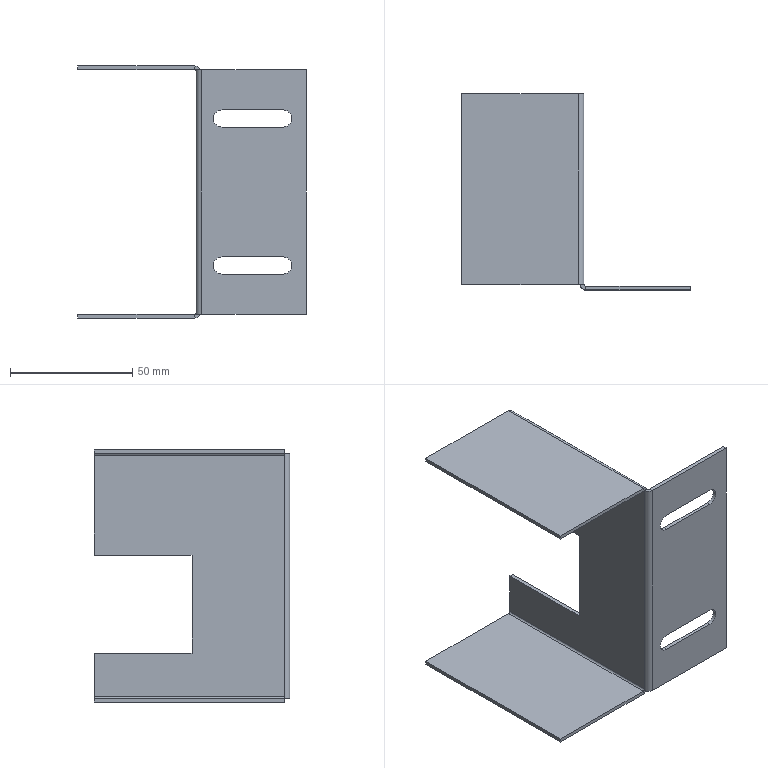Part | STEP file | Guide wheel mechanism revised.sldasm-Part-194 | 1 solid | 44 faces | box 93.5 x 80 x 103 mm | volume 26904 mm3 | plane 34 | cylinder 10 | commonest cylinder face diameters 7 x4 1.473 x3 4.473 x3
STEP:
#1=CARTESIAN_POINT('',(0.,80.,8.5));
#2=VERTEX_POINT('',#1);
#3=CARTESIAN_POINT('',(1.5,80.,8.5));
#4=VERTEX_POINT('',#3);
#5=CARTESIAN_POINT('',(0.,80.,8.5));
#6=DIRECTION('',(1.,0.,0.));
#7=VECTOR('',#6,1000.);
#8=LINE('',#5,#7);
#9=EDGE_CURVE('',#2,#4,#8,.T.);
#10=ORIENTED_EDGE('',*,*,#9,.F.);
#11=CARTESIAN_POINT('',(0.,80.,49.263));
#12=VERTEX_POINT('',#11);
#13=CARTESIAN_POINT('',(0.,80.,50.));
#14=DIRECTION('',(0.,0.,-1.));
#15=VECTOR('',#14,1000.);
#16=LINE('',#13,#15);
#17=EDGE_CURVE('',#12,#2,#16,.T.);
#18=ORIENTED_EDGE('',*,*,#17,.F.);
#19=CARTESIAN_POINT('',(1.5,80.,49.263));
#20=VERTEX_POINT('',#19);
#21=CARTESIAN_POINT('',(0.,80.,49.263));
#22=DIRECTION('',(1.,0.,0.));
#23=VECTOR('',#22,1000.);
#24=LINE('',#21,#23);
#25=EDGE_CURVE('',#12,#20,#24,.T.);
#26=ORIENTED_EDGE('',*,*,#25,.T.);
#27=CARTESIAN_POINT('',(1.5,80.,50.));
#28=DIRECTION('',(0.,0.,-1.));
#29=VECTOR('',#28,1000.);
#30=LINE('',#27,#29);
#31=EDGE_CURVE('',#20,#4,#30,.T.);
#32=ORIENTED_EDGE('',*,*,#31,.T.);
#33=EDGE_LOOP('',(#10,#18,#26,#32));
#34=FACE_OUTER_BOUND('',#33,.T.);
#35=CARTESIAN_POINT('',(0.,80.,50.));
#36=DIRECTION('',(0.,1.,0.));
#37=DIRECTION('',(0.,0.,1.));
#38=AXIS2_PLACEMENT_3D('',#35,#36,#37);
#39=PLANE('',#38);
#40=ADVANCED_FACE('',(#34),#39,.T.);
#41=CARTESIAN_POINT('',(1.5,2.237,50.));
#42=VERTEX_POINT('',#41);
#43=CARTESIAN_POINT('',(1.5,2.237,49.263));
#44=VERTEX_POINT('',#43);
#45=CARTESIAN_POINT('',(1.5,2.237,50.));
#46=DIRECTION('',(0.,0.,-1.));
#47=VECTOR('',#46,1000.);
#48=LINE('',#45,#47);
#49=EDGE_CURVE('',#42,#44,#48,.T.);
#50=ORIENTED_EDGE('',*,*,#49,.T.);
#51=CARTESIAN_POINT('',(1.375,2.237,50.));
#52=VERTEX_POINT('',#51);
#53=CARTESIAN_POINT('',(-0.7366,2.237,49.263));
#54=DIRECTION('',(0.,-1.,0.));
#55=DIRECTION('',(1.,0.,0.));
#56=AXIS2_PLACEMENT_3D('',#53,#54,#55);
#57=CIRCLE('',#56,2.237);
#58=EDGE_CURVE('',#44,#52,#57,.T.);
#59=ORIENTED_EDGE('',*,*,#58,.T.);
#60=CARTESIAN_POINT('',(0.,2.237,50.));
#61=DIRECTION('',(1.,0.,0.));
#62=VECTOR('',#61,1000.);
#63=LINE('',#60,#62);
#64=EDGE_CURVE('',#52,#42,#63,.T.);
#65=ORIENTED_EDGE('',*,*,#64,.T.);
#66=EDGE_LOOP('',(#50,#59,#65));
#67=FACE_OUTER_BOUND('',#66,.T.);
#68=CARTESIAN_POINT('',(0.,2.237,50.));
#69=DIRECTION('',(0.,-1.,0.));
#70=DIRECTION('',(1.,0.,0.));
#71=AXIS2_PLACEMENT_3D('',#68,#69,#70);
#72=PLANE('',#71);
#73=ADVANCED_FACE('',(#67),#72,.F.);
#74=CARTESIAN_POINT('',(1.5,40.,8.5));
#75=VERTEX_POINT('',#74);
#76=CARTESIAN_POINT('',(1.5,80.,8.5));
#77=DIRECTION('',(0.,-1.,0.));
#78=VECTOR('',#77,1000.);
#79=LINE('',#76,#78);
#80=EDGE_CURVE('',#4,#75,#79,.T.);
#81=ORIENTED_EDGE('',*,*,#80,.F.);
#82=ORIENTED_EDGE('',*,*,#31,.F.);
#83=CARTESIAN_POINT('',(1.5,468.817,49.263));
#84=DIRECTION('',(0.,-1.,0.));
#85=VECTOR('',#84,1000.);
#86=LINE('',#83,#85);
#87=EDGE_CURVE('',#20,#44,#86,.T.);
#88=ORIENTED_EDGE('',*,*,#87,.T.);
#89=CARTESIAN_POINT('',(1.5,2.237,-49.263));
#90=VERTEX_POINT('',#89);
#91=CARTESIAN_POINT('',(1.5,2.237,50.));
#92=DIRECTION('',(0.,0.,-1.));
#93=VECTOR('',#92,1000.);
#94=LINE('',#91,#93);
#95=EDGE_CURVE('',#44,#90,#94,.T.);
#96=ORIENTED_EDGE('',*,*,#95,.T.);
#97=CARTESIAN_POINT('',(1.5,80.,-49.263));
#98=VERTEX_POINT('',#97);
#99=CARTESIAN_POINT('',(1.5,2.237,-49.263));
#100=DIRECTION('',(0.,1.,0.));
#101=VECTOR('',#100,1000.);
#102=LINE('',#99,#101);
#103=EDGE_CURVE('',#90,#98,#102,.T.);
#104=ORIENTED_EDGE('',*,*,#103,.T.);
#105=CARTESIAN_POINT('',(1.5,80.,-31.5));
#106=VERTEX_POINT('',#105);
#107=CARTESIAN_POINT('',(1.5,80.,50.));
#108=DIRECTION('',(0.,0.,-1.));
#109=VECTOR('',#108,1000.);
#110=LINE('',#107,#109);
#111=EDGE_CURVE('',#106,#98,#110,.T.);
#112=ORIENTED_EDGE('',*,*,#111,.F.);
#113=CARTESIAN_POINT('',(1.5,40.,-31.5));
#114=VERTEX_POINT('',#113);
#115=CARTESIAN_POINT('',(1.5,80.,-31.5));
#116=DIRECTION('',(0.,1.,0.));
#117=VECTOR('',#116,1000.);
#118=LINE('',#115,#117);
#119=EDGE_CURVE('',#114,#106,#118,.T.);
#120=ORIENTED_EDGE('',*,*,#119,.F.);
#121=CARTESIAN_POINT('',(1.5,40.,8.5));
#122=DIRECTION('',(0.,0.,-1.));
#123=VECTOR('',#122,1000.);
#124=LINE('',#121,#123);
#125=EDGE_CURVE('',#75,#114,#124,.T.);
#126=ORIENTED_EDGE('',*,*,#125,.F.);
#127=EDGE_LOOP('',(#81,#82,#88,#96,#104,#112,#120,#126));
#128=FACE_OUTER_BOUND('',#127,.T.);
#129=CARTESIAN_POINT('',(1.5,80.,50.));
#130=DIRECTION('',(1.,0.,0.));
#131=DIRECTION('',(0.,1.,0.));
#132=AXIS2_PLACEMENT_3D('',#129,#130,#131);
#133=PLANE('',#132);
#134=ADVANCED_FACE('',(#128),#133,.T.);
#135=ORIENTED_EDGE('',*,*,#17,.T.);
#136=CARTESIAN_POINT('',(0.,40.,8.5));
#137=VERTEX_POINT('',#136);
#138=CARTESIAN_POINT('',(0.,80.,8.5));
#139=DIRECTION('',(0.,-1.,0.));
#140=VECTOR('',#139,1000.);
#141=LINE('',#138,#140);
#142=EDGE_CURVE('',#2,#137,#141,.T.);
#143=ORIENTED_EDGE('',*,*,#142,.T.);
#144=CARTESIAN_POINT('',(0.,40.,-31.5));
#145=VERTEX_POINT('',#144);
#146=CARTESIAN_POINT('',(0.,40.,50.));
#147=DIRECTION('',(0.,0.,-1.));
#148=VECTOR('',#147,1000.);
#149=LINE('',#146,#148);
#150=EDGE_CURVE('',#137,#145,#149,.T.);
#151=ORIENTED_EDGE('',*,*,#150,.T.);
#152=CARTESIAN_POINT('',(0.,80.,-31.5));
#153=VERTEX_POINT('',#152);
#154=CARTESIAN_POINT('',(0.,80.,-31.5));
#155=DIRECTION('',(0.,1.,0.));
#156=VECTOR('',#155,1000.);
#157=LINE('',#154,#156);
#158=EDGE_CURVE('',#145,#153,#157,.T.);
#159=ORIENTED_EDGE('',*,*,#158,.T.);
#160=CARTESIAN_POINT('',(0.,80.,-49.263));
#161=VERTEX_POINT('',#160);
#162=CARTESIAN_POINT('',(0.,80.,50.));
#163=DIRECTION('',(0.,0.,-1.));
#164=VECTOR('',#163,1000.);
#165=LINE('',#162,#164);
#166=EDGE_CURVE('',#153,#161,#165,.T.);
#167=ORIENTED_EDGE('',*,*,#166,.T.);
#168=CARTESIAN_POINT('',(0.,2.237,-49.263));
#169=VERTEX_POINT('',#168);
#170=CARTESIAN_POINT('',(0.,2.237,-49.263));
#171=DIRECTION('',(0.,1.,0.));
#172=VECTOR('',#171,1000.);
#173=LINE('',#170,#172);
#174=EDGE_CURVE('',#169,#161,#173,.T.);
#175=ORIENTED_EDGE('',*,*,#174,.F.);
#176=CARTESIAN_POINT('',(0.,2.237,49.263));
#177=VERTEX_POINT('',#176);
#178=CARTESIAN_POINT('',(0.,2.237,50.));
#179=DIRECTION('',(0.,0.,-1.));
#180=VECTOR('',#179,1000.);
#181=LINE('',#178,#180);
#182=EDGE_CURVE('',#177,#169,#181,.T.);
#183=ORIENTED_EDGE('',*,*,#182,.F.);
#184=CARTESIAN_POINT('',(0.,468.817,49.263));
#185=DIRECTION('',(0.,-1.,0.));
#186=VECTOR('',#185,1000.);
#187=LINE('',#184,#186);
#188=EDGE_CURVE('',#12,#177,#187,.T.);
#189=ORIENTED_EDGE('',*,*,#188,.F.);
#190=EDGE_LOOP('',(#135,#143,#151,#159,#167,#175,#183,#189));
#191=FACE_OUTER_BOUND('',#190,.T.);
#192=CARTESIAN_POINT('',(0.,80.,50.));
#193=DIRECTION('',(1.,0.,0.));
#194=DIRECTION('',(0.,1.,0.));
#195=AXIS2_PLACEMENT_3D('',#192,#193,#194);
#196=PLANE('',#195);
#197=ADVANCED_FACE('',(#191),#196,.F.);
#198=CARTESIAN_POINT('',(0.,80.,-31.5));
#199=DIRECTION('',(-1.,0.,0.));
#200=VECTOR('',#199,1000.);
#201=LINE('',#198,#200);
#202=EDGE_CURVE('',#106,#153,#201,.T.);
#203=ORIENTED_EDGE('',*,*,#202,.F.);
#204=ORIENTED_EDGE('',*,*,#111,.T.);
#205=CARTESIAN_POINT('',(0.,80.,-49.263));
#206=DIRECTION('',(1.,0.,0.));
#207=VECTOR('',#206,1000.);
#208=LINE('',#205,#207);
#209=EDGE_CURVE('',#161,#98,#208,.T.);
#210=ORIENTED_EDGE('',*,*,#209,.F.);
#211=ORIENTED_EDGE('',*,*,#166,.F.);
#212=EDGE_LOOP('',(#203,#204,#210,#211));
#213=FACE_OUTER_BOUND('',#212,.T.);
#214=CARTESIAN_POINT('',(0.,80.,50.));
#215=DIRECTION('',(0.,1.,0.));
#216=DIRECTION('',(0.,0.,1.));
#217=AXIS2_PLACEMENT_3D('',#214,#215,#216);
#218=PLANE('',#217);
#219=ADVANCED_FACE('',(#213),#218,.T.);
#220=CARTESIAN_POINT('',(1.5,2.237,-50.));
#221=VERTEX_POINT('',#220);
#222=CARTESIAN_POINT('',(1.375,2.237,-50.));
#223=VERTEX_POINT('',#222);
#224=CARTESIAN_POINT('',(1.5,2.237,-50.));
#225=DIRECTION('',(-1.,0.,0.));
#226=VECTOR('',#225,1000.);
#227=LINE('',#224,#226);
#228=EDGE_CURVE('',#221,#223,#227,.T.);
#229=ORIENTED_EDGE('',*,*,#228,.T.);
#230=CARTESIAN_POINT('',(-0.7366,2.237,-49.263));
#231=DIRECTION('',(0.,-1.,0.));
#232=DIRECTION('',(1.,0.,0.));
#233=AXIS2_PLACEMENT_3D('',#230,#231,#232);
#234=CIRCLE('',#233,2.237);
#235=EDGE_CURVE('',#223,#90,#234,.T.);
#236=ORIENTED_EDGE('',*,*,#235,.T.);
#237=CARTESIAN_POINT('',(1.5,2.237,50.));
#238=DIRECTION('',(0.,0.,1.));
#239=VECTOR('',#238,1000.);
#240=LINE('',#237,#239);
#241=EDGE_CURVE('',#221,#90,#240,.T.);
#242=ORIENTED_EDGE('',*,*,#241,.F.);
#243=EDGE_LOOP('',(#229,#236,#242));
#244=FACE_OUTER_BOUND('',#243,.T.);
#245=CARTESIAN_POINT('',(0.,2.237,-50.));
#246=DIRECTION('',(0.,1.,0.));
#247=DIRECTION('',(-1.,0.,0.));
#248=AXIS2_PLACEMENT_3D('',#245,#246,#247);
#249=PLANE('',#248);
#250=ADVANCED_FACE('',(#244),#249,.T.);
#251=CARTESIAN_POINT('',(2.237,0.,-50.));
#252=VERTEX_POINT('',#251);
#253=CARTESIAN_POINT('',(45.,0.,-50.));
#254=VERTEX_POINT('',#253);
#255=CARTESIAN_POINT('',(0.,0.,-50.));
#256=DIRECTION('',(1.,0.,0.));
#257=VECTOR('',#256,1000.);
#258=LINE('',#255,#257);
#259=EDGE_CURVE('',#252,#254,#258,.T.);
#260=ORIENTED_EDGE('',*,*,#259,.T.);
#261=CARTESIAN_POINT('',(45.,0.,50.));
#262=VERTEX_POINT('',#261);
#263=CARTESIAN_POINT('',(45.,0.,50.));
#264=DIRECTION('',(0.,0.,-1.));
#265=VECTOR('',#264,1000.);
#266=LINE('',#263,#265);
#267=EDGE_CURVE('',#262,#254,#266,.T.);
#268=ORIENTED_EDGE('',*,*,#267,.F.);
#269=CARTESIAN_POINT('',(2.237,0.,50.));
#270=VERTEX_POINT('',#269);
#271=CARTESIAN_POINT('',(0.,0.,50.));
#272=DIRECTION('',(1.,0.,0.));
#273=VECTOR('',#272,1000.);
#274=LINE('',#271,#273);
#275=EDGE_CURVE('',#270,#262,#274,.T.);
#276=ORIENTED_EDGE('',*,*,#275,.F.);
#277=CARTESIAN_POINT('',(2.237,0.,50.));
#278=DIRECTION('',(0.,0.,-1.));
#279=VECTOR('',#278,1000.);
#280=LINE('',#277,#279);
#281=EDGE_CURVE('',#270,#252,#280,.T.);
#282=ORIENTED_EDGE('',*,*,#281,.T.);
#283=EDGE_LOOP('',(#260,#268,#276,#282));
#284=FACE_OUTER_BOUND('',#283,.T.);
#285=CARTESIAN_POINT('',(35.5,0.,-33.5));
#286=VERTEX_POINT('',#285);
#287=CARTESIAN_POINT('',(10.5,0.,-33.5));
#288=VERTEX_POINT('',#287);
#289=CARTESIAN_POINT('',(0.,0.,-33.5));
#290=DIRECTION('',(-1.,0.,0.));
#291=VECTOR('',#290,1000.);
#292=LINE('',#289,#291);
#293=EDGE_CURVE('',#286,#288,#292,.T.);
#294=ORIENTED_EDGE('',*,*,#293,.T.);
#295=CARTESIAN_POINT('',(10.5,0.,-26.5));
#296=VERTEX_POINT('',#295);
#297=CARTESIAN_POINT('',(10.5,0.,-30.));
#298=DIRECTION('',(0.,1.,0.));
#299=DIRECTION('',(0.,0.,1.));
#300=AXIS2_PLACEMENT_3D('',#297,#298,#299);
#301=CIRCLE('',#300,3.5);
#302=EDGE_CURVE('',#288,#296,#301,.T.);
#303=ORIENTED_EDGE('',*,*,#302,.T.);
#304=CARTESIAN_POINT('',(35.5,0.,-26.5));
#305=VERTEX_POINT('',#304);
#306=CARTESIAN_POINT('',(0.,0.,-26.5));
#307=DIRECTION('',(1.,0.,0.));
#308=VECTOR('',#307,1000.);
#309=LINE('',#306,#308);
#310=EDGE_CURVE('',#296,#305,#309,.T.);
#311=ORIENTED_EDGE('',*,*,#310,.T.);
#312=CARTESIAN_POINT('',(35.5,0.,-30.));
#313=DIRECTION('',(0.,1.,0.));
#314=DIRECTION('',(0.,0.,1.));
#315=AXIS2_PLACEMENT_3D('',#312,#313,#314);
#316=CIRCLE('',#315,3.5);
#317=EDGE_CURVE('',#305,#286,#316,.T.);
#318=ORIENTED_EDGE('',*,*,#317,.T.);
#319=EDGE_LOOP('',(#294,#303,#311,#318));
#320=FACE_BOUND('',#319,.T.);
#321=CARTESIAN_POINT('',(10.5,0.,33.5));
#322=VERTEX_POINT('',#321);
#323=CARTESIAN_POINT('',(10.5,0.,26.5));
#324=VERTEX_POINT('',#323);
#325=CARTESIAN_POINT('',(10.5,0.,30.));
#326=DIRECTION('',(0.,-1.,0.));
#327=DIRECTION('',(0.,0.,1.));
#328=AXIS2_PLACEMENT_3D('',#325,#326,#327);
#329=CIRCLE('',#328,3.5);
#330=EDGE_CURVE('',#322,#324,#329,.T.);
#331=ORIENTED_EDGE('',*,*,#330,.F.);
#332=CARTESIAN_POINT('',(35.5,0.,33.5));
#333=VERTEX_POINT('',#332);
#334=CARTESIAN_POINT('',(0.,0.,33.5));
#335=DIRECTION('',(-1.,0.,0.));
#336=VECTOR('',#335,1000.);
#337=LINE('',#334,#336);
#338=EDGE_CURVE('',#333,#322,#337,.T.);
#339=ORIENTED_EDGE('',*,*,#338,.F.);
#340=CARTESIAN_POINT('',(35.5,0.,26.5));
#341=VERTEX_POINT('',#340);
#342=CARTESIAN_POINT('',(35.5,0.,30.));
#343=DIRECTION('',(0.,-1.,0.));
#344=DIRECTION('',(0.,0.,1.));
#345=AXIS2_PLACEMENT_3D('',#342,#343,#344);
#346=CIRCLE('',#345,3.5);
#347=EDGE_CURVE('',#341,#333,#346,.T.);
#348=ORIENTED_EDGE('',*,*,#347,.F.);
#349=CARTESIAN_POINT('',(0.,0.,26.5));
#350=DIRECTION('',(1.,0.,0.));
#351=VECTOR('',#350,1000.);
#352=LINE('',#349,#351);
#353=EDGE_CURVE('',#324,#341,#352,.T.);
#354=ORIENTED_EDGE('',*,*,#353,.F.);
#355=EDGE_LOOP('',(#331,#339,#348,#354));
#356=FACE_BOUND('',#355,.T.);
#357=CARTESIAN_POINT('',(0.,0.,50.));
#358=DIRECTION('',(0.,1.,0.));
#359=DIRECTION('',(0.,0.,1.));
#360=AXIS2_PLACEMENT_3D('',#357,#358,#359);
#361=PLANE('',#360);
#362=ADVANCED_FACE('',(#284,#320,#356),#361,.F.);
#363=CARTESIAN_POINT('',(2.237,1.5,-50.));
#364=VERTEX_POINT('',#363);
#365=CARTESIAN_POINT('',(45.,1.5,-50.));
#366=VERTEX_POINT('',#365);
#367=CARTESIAN_POINT('',(0.,1.5,-50.));
#368=DIRECTION('',(1.,0.,0.));
#369=VECTOR('',#368,1000.);
#370=LINE('',#367,#369);
#371=EDGE_CURVE('',#364,#366,#370,.T.);
#372=ORIENTED_EDGE('',*,*,#371,.F.);
#373=CARTESIAN_POINT('',(2.237,1.5,50.));
#374=VERTEX_POINT('',#373);
#375=CARTESIAN_POINT('',(2.237,1.5,50.));
#376=DIRECTION('',(0.,0.,-1.));
#377=VECTOR('',#376,1000.);
#378=LINE('',#375,#377);
#379=EDGE_CURVE('',#374,#364,#378,.T.);
#380=ORIENTED_EDGE('',*,*,#379,.F.);
#381=CARTESIAN_POINT('',(45.,1.5,50.));
#382=VERTEX_POINT('',#381);
#383=CARTESIAN_POINT('',(0.,1.5,50.));
#384=DIRECTION('',(1.,0.,0.));
#385=VECTOR('',#384,1000.);
#386=LINE('',#383,#385);
#387=EDGE_CURVE('',#374,#382,#386,.T.);
#388=ORIENTED_EDGE('',*,*,#387,.T.);
#389=CARTESIAN_POINT('',(45.,1.5,50.));
#390=DIRECTION('',(0.,0.,-1.));
#391=VECTOR('',#390,1000.);
#392=LINE('',#389,#391);
#393=EDGE_CURVE('',#382,#366,#392,.T.);
#394=ORIENTED_EDGE('',*,*,#393,.T.);
#395=EDGE_LOOP('',(#372,#380,#388,#394));
#396=FACE_OUTER_BOUND('',#395,.T.);
#397=CARTESIAN_POINT('',(10.5,1.5,-33.5));
#398=VERTEX_POINT('',#397);
#399=CARTESIAN_POINT('',(10.5,1.5,-26.5));
#400=VERTEX_POINT('',#399);
#401=CARTESIAN_POINT('',(10.5,1.5,-30.));
#402=DIRECTION('',(0.,1.,0.));
#403=DIRECTION('',(0.,0.,1.));
#404=AXIS2_PLACEMENT_3D('',#401,#402,#403);
#405=CIRCLE('',#404,3.5);
#406=EDGE_CURVE('',#398,#400,#405,.T.);
#407=ORIENTED_EDGE('',*,*,#406,.F.);
#408=CARTESIAN_POINT('',(35.5,1.5,-33.5));
#409=VERTEX_POINT('',#408);
#410=CARTESIAN_POINT('',(10.5,1.5,-33.5));
#411=DIRECTION('',(-1.,0.,0.));
#412=VECTOR('',#411,1000.);
#413=LINE('',#410,#412);
#414=EDGE_CURVE('',#409,#398,#413,.T.);
#415=ORIENTED_EDGE('',*,*,#414,.F.);
#416=CARTESIAN_POINT('',(35.5,1.5,-26.5));
#417=VERTEX_POINT('',#416);
#418=CARTESIAN_POINT('',(35.5,1.5,-30.));
#419=DIRECTION('',(0.,1.,0.));
#420=DIRECTION('',(0.,0.,1.));
#421=AXIS2_PLACEMENT_3D('',#418,#419,#420);
#422=CIRCLE('',#421,3.5);
#423=EDGE_CURVE('',#417,#409,#422,.T.);
#424=ORIENTED_EDGE('',*,*,#423,.F.);
#425=CARTESIAN_POINT('',(10.5,1.5,-26.5));
#426=DIRECTION('',(1.,0.,0.));
#427=VECTOR('',#426,1000.);
#428=LINE('',#425,#427);
#429=EDGE_CURVE('',#400,#417,#428,.T.);
#430=ORIENTED_EDGE('',*,*,#429,.F.);
#431=EDGE_LOOP('',(#407,#415,#424,#430));
#432=FACE_BOUND('',#431,.T.);
#433=CARTESIAN_POINT('',(35.5,1.5,33.5));
#434=VERTEX_POINT('',#433);
#435=CARTESIAN_POINT('',(10.5,1.5,33.5));
#436=VERTEX_POINT('',#435);
#437=CARTESIAN_POINT('',(10.5,1.5,33.5));
#438=DIRECTION('',(-1.,0.,0.));
#439=VECTOR('',#438,1000.);
#440=LINE('',#437,#439);
#441=EDGE_CURVE('',#434,#436,#440,.T.);
#442=ORIENTED_EDGE('',*,*,#441,.T.);
#443=CARTESIAN_POINT('',(10.5,1.5,26.5));
#444=VERTEX_POINT('',#443);
#445=CARTESIAN_POINT('',(10.5,1.5,30.));
#446=DIRECTION('',(0.,-1.,0.));
#447=DIRECTION('',(0.,0.,-1.));
#448=AXIS2_PLACEMENT_3D('',#445,#446,#447);
#449=CIRCLE('',#448,3.5);
#450=EDGE_CURVE('',#436,#444,#449,.T.);
#451=ORIENTED_EDGE('',*,*,#450,.T.);
#452=CARTESIAN_POINT('',(35.5,1.5,26.5));
#453=VERTEX_POINT('',#452);
#454=CARTESIAN_POINT('',(10.5,1.5,26.5));
#455=DIRECTION('',(1.,0.,0.));
#456=VECTOR('',#455,1000.);
#457=LINE('',#454,#456);
#458=EDGE_CURVE('',#444,#453,#457,.T.);
#459=ORIENTED_EDGE('',*,*,#458,.T.);
#460=CARTESIAN_POINT('',(35.5,1.5,30.));
#461=DIRECTION('',(0.,-1.,0.));
#462=DIRECTION('',(0.,0.,-1.));
#463=AXIS2_PLACEMENT_3D('',#460,#461,#462);
#464=CIRCLE('',#463,3.5);
#465=EDGE_CURVE('',#453,#434,#464,.T.);
#466=ORIENTED_EDGE('',*,*,#465,.T.);
#467=EDGE_LOOP('',(#442,#451,#459,#466));
#468=FACE_BOUND('',#467,.T.);
#469=CARTESIAN_POINT('',(0.,1.5,50.));
#470=DIRECTION('',(0.,1.,0.));
#471=DIRECTION('',(0.,0.,1.));
#472=AXIS2_PLACEMENT_3D('',#469,#470,#471);
#473=PLANE('',#472);
#474=ADVANCED_FACE('',(#396,#432,#468),#473,.T.);
#475=CARTESIAN_POINT('',(0.,2.237,50.));
#476=VERTEX_POINT('',#475);
#477=CARTESIAN_POINT('',(0.,2.237,50.));
#478=DIRECTION('',(1.,0.,0.));
#479=VECTOR('',#478,1000.);
#480=LINE('',#477,#479);
#481=EDGE_CURVE('',#476,#52,#480,.T.);
#482=ORIENTED_EDGE('',*,*,#481,.F.);
#483=CARTESIAN_POINT('',(2.237,2.237,50.));
#484=DIRECTION('',(0.,0.,1.));
#485=DIRECTION('',(-1.,0.,0.));
#486=AXIS2_PLACEMENT_3D('',#483,#484,#485);
#487=CIRCLE('',#486,2.237);
#488=EDGE_CURVE('',#476,#270,#487,.T.);
#489=ORIENTED_EDGE('',*,*,#488,.T.);
#490=CARTESIAN_POINT('',(2.237,1.5,50.));
#491=DIRECTION('',(0.,-1.,0.));
#492=VECTOR('',#491,1000.);
#493=LINE('',#490,#492);
#494=EDGE_CURVE('',#374,#270,#493,.T.);
#495=ORIENTED_EDGE('',*,*,#494,.F.);
#496=CARTESIAN_POINT('',(2.237,2.237,50.));
#497=DIRECTION('',(0.,0.,1.));
#498=DIRECTION('',(1.,0.,0.));
#499=AXIS2_PLACEMENT_3D('',#496,#497,#498);
#500=CIRCLE('',#499,0.7366);
#501=EDGE_CURVE('',#42,#374,#500,.T.);
#502=ORIENTED_EDGE('',*,*,#501,.F.);
#503=ORIENTED_EDGE('',*,*,#64,.F.);
#504=EDGE_LOOP('',(#482,#489,#495,#502,#503));
#505=FACE_OUTER_BOUND('',#504,.T.);
#506=CARTESIAN_POINT('',(0.,2.237,50.));
#507=DIRECTION('',(0.,0.,1.));
#508=DIRECTION('',(1.,0.,0.));
#509=AXIS2_PLACEMENT_3D('',#506,#507,#508);
#510=PLANE('',#509);
#511=ADVANCED_FACE('',(#505),#510,.T.);
#512=CARTESIAN_POINT('',(2.237,0.,-50.));
#513=DIRECTION('',(0.,1.,0.));
#514=VECTOR('',#513,1000.);
#515=LINE('',#512,#514);
#516=EDGE_CURVE('',#252,#364,#515,.T.);
#517=ORIENTED_EDGE('',*,*,#516,.F.);
#518=CARTESIAN_POINT('',(0.,2.237,-50.));
#519=VERTEX_POINT('',#518);
#520=CARTESIAN_POINT('',(2.237,2.237,-50.));
#521=DIRECTION('',(0.,0.,1.));
#522=DIRECTION('',(-1.,0.,0.));
#523=AXIS2_PLACEMENT_3D('',#520,#521,#522);
#524=CIRCLE('',#523,2.237);
#525=EDGE_CURVE('',#519,#252,#524,.T.);
#526=ORIENTED_EDGE('',*,*,#525,.F.);
#527=CARTESIAN_POINT('',(1.5,2.237,-50.));
#528=DIRECTION('',(-1.,0.,0.));
#529=VECTOR('',#528,1000.);
#530=LINE('',#527,#529);
#531=EDGE_CURVE('',#223,#519,#530,.T.);
#532=ORIENTED_EDGE('',*,*,#531,.F.);
#533=ORIENTED_EDGE('',*,*,#228,.F.);
#534=CARTESIAN_POINT('',(2.237,2.237,-50.));
#535=DIRECTION('',(0.,0.,1.));
#536=DIRECTION('',(1.,0.,0.));
#537=AXIS2_PLACEMENT_3D('',#534,#535,#536);
#538=CIRCLE('',#537,0.7366);
#539=EDGE_CURVE('',#221,#364,#538,.T.);
#540=ORIENTED_EDGE('',*,*,#539,.T.);
#541=EDGE_LOOP('',(#517,#526,#532,#533,#540));
#542=FACE_OUTER_BOUND('',#541,.T.);
#543=CARTESIAN_POINT('',(2.237,0.,-50.));
#544=DIRECTION('',(0.,0.,-1.));
#545=DIRECTION('',(-1.,0.,0.));
#546=AXIS2_PLACEMENT_3D('',#543,#544,#545);
#547=PLANE('',#546);
#548=ADVANCED_FACE('',(#542),#547,.T.);
#549=ORIENTED_EDGE('',*,*,#259,.F.);
#550=ORIENTED_EDGE('',*,*,#516,.T.);
#551=ORIENTED_EDGE('',*,*,#371,.T.);
#552=CARTESIAN_POINT('',(45.,1.5,-50.));
#553=DIRECTION('',(0.,-1.,0.));
#554=VECTOR('',#553,1000.);
#555=LINE('',#552,#554);
#556=EDGE_CURVE('',#366,#254,#555,.T.);
#557=ORIENTED_EDGE('',*,*,#556,.T.);
#558=EDGE_LOOP('',(#549,#550,#551,#557));
#559=FACE_OUTER_BOUND('',#558,.T.);
#560=CARTESIAN_POINT('',(1.5,2.237,-50.));
#561=DIRECTION('',(0.,0.,-1.));
#562=DIRECTION('',(-1.,0.,0.));
#563=AXIS2_PLACEMENT_3D('',#560,#561,#562);
#564=PLANE('',#563);
#565=ADVANCED_FACE('',(#559),#564,.T.);
#566=ORIENTED_EDGE('',*,*,#556,.F.);
#567=ORIENTED_EDGE('',*,*,#393,.F.);
#568=CARTESIAN_POINT('',(45.,1.5,50.));
#569=DIRECTION('',(0.,-1.,0.));
#570=VECTOR('',#569,1000.);
#571=LINE('',#568,#570);
#572=EDGE_CURVE('',#382,#262,#571,.T.);
#573=ORIENTED_EDGE('',*,*,#572,.T.);
#574=ORIENTED_EDGE('',*,*,#267,.T.);
#575=EDGE_LOOP('',(#566,#567,#573,#574));
#576=FACE_OUTER_BOUND('',#575,.T.);
#577=CARTESIAN_POINT('',(45.,1.5,50.));
#578=DIRECTION('',(1.,0.,0.));
#579=DIRECTION('',(0.,0.,-1.));
#580=AXIS2_PLACEMENT_3D('',#577,#578,#579);
#581=PLANE('',#580);
#582=ADVANCED_FACE('',(#576),#581,.T.);
#583=ORIENTED_EDGE('',*,*,#539,.F.);
#584=ORIENTED_EDGE('',*,*,#241,.T.);
#585=ORIENTED_EDGE('',*,*,#95,.F.);
#586=ORIENTED_EDGE('',*,*,#49,.F.);
#587=ORIENTED_EDGE('',*,*,#501,.T.);
#588=ORIENTED_EDGE('',*,*,#379,.T.);
#589=EDGE_LOOP('',(#583,#584,#585,#586,#587,#588));
#590=FACE_OUTER_BOUND('',#589,.T.);
#591=CARTESIAN_POINT('',(2.237,2.237,50.));
#592=DIRECTION('',(0.,0.,-1.));
#593=DIRECTION('',(-1.,0.,0.));
#594=AXIS2_PLACEMENT_3D('',#591,#592,#593);
#595=CYLINDRICAL_SURFACE('',#594,0.7366);
#596=ADVANCED_FACE('',(#590),#595,.F.);
#597=ORIENTED_EDGE('',*,*,#525,.T.);
#598=ORIENTED_EDGE('',*,*,#281,.F.);
#599=ORIENTED_EDGE('',*,*,#488,.F.);
#600=CARTESIAN_POINT('',(0.,2.237,50.));
#601=DIRECTION('',(0.,0.,-1.));
#602=VECTOR('',#601,1000.);
#603=LINE('',#600,#602);
#604=EDGE_CURVE('',#476,#177,#603,.T.);
#605=ORIENTED_EDGE('',*,*,#604,.T.);
#606=ORIENTED_EDGE('',*,*,#182,.T.);
#607=CARTESIAN_POINT('',(0.,2.237,-50.));
#608=DIRECTION('',(0.,0.,1.));
#609=VECTOR('',#608,1000.);
#610=LINE('',#607,#609);
#611=EDGE_CURVE('',#519,#169,#610,.T.);
#612=ORIENTED_EDGE('',*,*,#611,.F.);
#613=EDGE_LOOP('',(#597,#598,#599,#605,#606,#612));
#614=FACE_OUTER_BOUND('',#613,.T.);
#615=CARTESIAN_POINT('',(2.237,2.237,50.));
#616=DIRECTION('',(0.,0.,-1.));
#617=DIRECTION('',(-1.,0.,0.));
#618=AXIS2_PLACEMENT_3D('',#615,#616,#617);
#619=CYLINDRICAL_SURFACE('',#618,2.237);
#620=ADVANCED_FACE('',(#614),#619,.T.);
#621=ORIENTED_EDGE('',*,*,#275,.T.);
#622=ORIENTED_EDGE('',*,*,#572,.F.);
#623=ORIENTED_EDGE('',*,*,#387,.F.);
#624=ORIENTED_EDGE('',*,*,#494,.T.);
#625=EDGE_LOOP('',(#621,#622,#623,#624));
#626=FACE_OUTER_BOUND('',#625,.T.);
#627=CARTESIAN_POINT('',(2.237,2.237,50.));
#628=DIRECTION('',(0.,0.,1.));
#629=DIRECTION('',(1.,0.,0.));
#630=AXIS2_PLACEMENT_3D('',#627,#628,#629);
#631=PLANE('',#630);
#632=ADVANCED_FACE('',(#626),#631,.T.);
#633=CARTESIAN_POINT('',(10.5,-8.5,-33.5));
#634=DIRECTION('',(0.,1.,0.));
#635=VECTOR('',#634,1000.);
#636=LINE('',#633,#635);
#637=EDGE_CURVE('',#288,#398,#636,.T.);
#638=ORIENTED_EDGE('',*,*,#637,.T.);
#639=ORIENTED_EDGE('',*,*,#406,.T.);
#640=CARTESIAN_POINT('',(10.5,-8.5,-26.5));
#641=DIRECTION('',(0.,1.,0.));
#642=VECTOR('',#641,1000.);
#643=LINE('',#640,#642);
#644=EDGE_CURVE('',#296,#400,#643,.T.);
#645=ORIENTED_EDGE('',*,*,#644,.F.);
#646=ORIENTED_EDGE('',*,*,#302,.F.);
#647=EDGE_LOOP('',(#638,#639,#645,#646));
#648=FACE_OUTER_BOUND('',#647,.T.);
#649=CARTESIAN_POINT('',(10.5,-8.5,-30.));
#650=DIRECTION('',(0.,1.,0.));
#651=DIRECTION('',(0.,0.,1.));
#652=AXIS2_PLACEMENT_3D('',#649,#650,#651);
#653=CYLINDRICAL_SURFACE('',#652,3.5);
#654=ADVANCED_FACE('',(#648),#653,.F.);
#655=CARTESIAN_POINT('',(35.5,-8.5,-33.5));
#656=DIRECTION('',(0.,1.,0.));
#657=VECTOR('',#656,1000.);
#658=LINE('',#655,#657);
#659=EDGE_CURVE('',#286,#409,#658,.T.);
#660=ORIENTED_EDGE('',*,*,#659,.T.);
#661=ORIENTED_EDGE('',*,*,#414,.T.);
#662=ORIENTED_EDGE('',*,*,#637,.F.);
#663=ORIENTED_EDGE('',*,*,#293,.F.);
#664=EDGE_LOOP('',(#660,#661,#662,#663));
#665=FACE_OUTER_BOUND('',#664,.T.);
#666=CARTESIAN_POINT('',(10.5,-8.5,-33.5));
#667=DIRECTION('',(0.,0.,-1.));
#668=DIRECTION('',(-1.,0.,0.));
#669=AXIS2_PLACEMENT_3D('',#666,#667,#668);
#670=PLANE('',#669);
#671=ADVANCED_FACE('',(#665),#670,.F.);
#672=CARTESIAN_POINT('',(35.5,-8.5,-26.5));
#673=DIRECTION('',(0.,1.,0.));
#674=VECTOR('',#673,1000.);
#675=LINE('',#672,#674);
#676=EDGE_CURVE('',#305,#417,#675,.T.);
#677=ORIENTED_EDGE('',*,*,#676,.T.);
#678=ORIENTED_EDGE('',*,*,#423,.T.);
#679=ORIENTED_EDGE('',*,*,#659,.F.);
#680=ORIENTED_EDGE('',*,*,#317,.F.);
#681=EDGE_LOOP('',(#677,#678,#679,#680));
#682=FACE_OUTER_BOUND('',#681,.T.);
#683=CARTESIAN_POINT('',(35.5,-8.5,-30.));
#684=DIRECTION('',(0.,1.,0.));
#685=DIRECTION('',(0.,0.,1.));
#686=AXIS2_PLACEMENT_3D('',#683,#684,#685);
#687=CYLINDRICAL_SURFACE('',#686,3.5);
#688=ADVANCED_FACE('',(#682),#687,.F.);
#689=ORIENTED_EDGE('',*,*,#644,.T.);
#690=ORIENTED_EDGE('',*,*,#429,.T.);
#691=ORIENTED_EDGE('',*,*,#676,.F.);
#692=ORIENTED_EDGE('',*,*,#310,.F.);
#693=EDGE_LOOP('',(#689,#690,#691,#692));
#694=FACE_OUTER_BOUND('',#693,.T.);
#695=CARTESIAN_POINT('',(10.5,-8.5,-26.5));
#696=DIRECTION('',(0.,0.,1.));
#697=DIRECTION('',(1.,0.,0.));
#698=AXIS2_PLACEMENT_3D('',#695,#696,#697);
#699=PLANE('',#698);
#700=ADVANCED_FACE('',(#694),#699,.F.);
#701=ORIENTED_EDGE('',*,*,#330,.T.);
#702=CARTESIAN_POINT('',(10.5,-8.5,26.5));
#703=DIRECTION('',(0.,1.,0.));
#704=VECTOR('',#703,1000.);
#705=LINE('',#702,#704);
#706=EDGE_CURVE('',#324,#444,#705,.T.);
#707=ORIENTED_EDGE('',*,*,#706,.T.);
#708=ORIENTED_EDGE('',*,*,#450,.F.);
#709=CARTESIAN_POINT('',(10.5,-8.5,33.5));
#710=DIRECTION('',(0.,1.,0.));
#711=VECTOR('',#710,1000.);
#712=LINE('',#709,#711);
#713=EDGE_CURVE('',#322,#436,#712,.T.);
#714=ORIENTED_EDGE('',*,*,#713,.F.);
#715=EDGE_LOOP('',(#701,#707,#708,#714));
#716=FACE_OUTER_BOUND('',#715,.T.);
#717=CARTESIAN_POINT('',(10.5,-8.5,30.));
#718=DIRECTION('',(0.,1.,0.));
#719=DIRECTION('',(0.,0.,1.));
#720=AXIS2_PLACEMENT_3D('',#717,#718,#719);
#721=CYLINDRICAL_SURFACE('',#720,3.5);
#722=ADVANCED_FACE('',(#716),#721,.F.);
#723=ORIENTED_EDGE('',*,*,#353,.T.);
#724=CARTESIAN_POINT('',(35.5,-8.5,26.5));
#725=DIRECTION('',(0.,1.,0.));
#726=VECTOR('',#725,1000.);
#727=LINE('',#724,#726);
#728=EDGE_CURVE('',#341,#453,#727,.T.);
#729=ORIENTED_EDGE('',*,*,#728,.T.);
#730=ORIENTED_EDGE('',*,*,#458,.F.);
#731=ORIENTED_EDGE('',*,*,#706,.F.);
#732=EDGE_LOOP('',(#723,#729,#730,#731));
#733=FACE_OUTER_BOUND('',#732,.T.);
#734=CARTESIAN_POINT('',(10.5,-8.5,26.5));
#735=DIRECTION('',(0.,0.,1.));
#736=DIRECTION('',(1.,0.,0.));
#737=AXIS2_PLACEMENT_3D('',#734,#735,#736);
#738=PLANE('',#737);
#739=ADVANCED_FACE('',(#733),#738,.T.);
#740=ORIENTED_EDGE('',*,*,#347,.T.);
#741=CARTESIAN_POINT('',(35.5,-8.5,33.5));
#742=DIRECTION('',(0.,1.,0.));
#743=VECTOR('',#742,1000.);
#744=LINE('',#741,#743);
#745=EDGE_CURVE('',#333,#434,#744,.T.);
#746=ORIENTED_EDGE('',*,*,#745,.T.);
#747=ORIENTED_EDGE('',*,*,#465,.F.);
#748=ORIENTED_EDGE('',*,*,#728,.F.);
#749=EDGE_LOOP('',(#740,#746,#747,#748));
#750=FACE_OUTER_BOUND('',#749,.T.);
#751=CARTESIAN_POINT('',(35.5,-8.5,30.));
#752=DIRECTION('',(0.,1.,0.));
#753=DIRECTION('',(0.,0.,1.));
#754=AXIS2_PLACEMENT_3D('',#751,#752,#753);
#755=CYLINDRICAL_SURFACE('',#754,3.5);
#756=ADVANCED_FACE('',(#750),#755,.F.);
#757=ORIENTED_EDGE('',*,*,#338,.T.);
#758=ORIENTED_EDGE('',*,*,#713,.T.);
#759=ORIENTED_EDGE('',*,*,#441,.F.);
#760=ORIENTED_EDGE('',*,*,#745,.F.);
#761=EDGE_LOOP('',(#757,#758,#759,#760));
#762=FACE_OUTER_BOUND('',#761,.T.);
#763=CARTESIAN_POINT('',(10.5,-8.5,33.5));
#764=DIRECTION('',(0.,0.,-1.));
#765=DIRECTION('',(-1.,0.,0.));
#766=AXIS2_PLACEMENT_3D('',#763,#764,#765);
#767=PLANE('',#766);
#768=ADVANCED_FACE('',(#762),#767,.T.);
#769=CARTESIAN_POINT('',(-0.7366,80.,-50.));
#770=VERTEX_POINT('',#769);
#771=CARTESIAN_POINT('',(-0.7366,80.,-51.5));
#772=VERTEX_POINT('',#771);
#773=CARTESIAN_POINT('',(-0.7366,80.,-50.));
#774=DIRECTION('',(0.,0.,-1.));
#775=VECTOR('',#774,1000.);
#776=LINE('',#773,#775);
#777=EDGE_CURVE('',#770,#772,#776,.T.);
#778=ORIENTED_EDGE('',*,*,#777,.F.);
#779=CARTESIAN_POINT('',(-0.7366,80.,-49.263));
#780=DIRECTION('',(0.,1.,0.));
#781=DIRECTION('',(1.,0.,0.));
#782=AXIS2_PLACEMENT_3D('',#779,#780,#781);
#783=CIRCLE('',#782,0.7366);
#784=EDGE_CURVE('',#161,#770,#783,.T.);
#785=ORIENTED_EDGE('',*,*,#784,.F.);
#786=ORIENTED_EDGE('',*,*,#209,.T.);
#787=CARTESIAN_POINT('',(-0.7366,80.,-49.263));
#788=DIRECTION('',(0.,1.,0.));
#789=DIRECTION('',(1.,0.,0.));
#790=AXIS2_PLACEMENT_3D('',#787,#788,#789);
#791=CIRCLE('',#790,2.237);
#792=EDGE_CURVE('',#98,#772,#791,.T.);
#793=ORIENTED_EDGE('',*,*,#792,.T.);
#794=EDGE_LOOP('',(#778,#785,#786,#793));
#795=FACE_OUTER_BOUND('',#794,.T.);
#796=CARTESIAN_POINT('',(-0.7366,80.,-49.263));
#797=DIRECTION('',(0.,1.,0.));
#798=DIRECTION('',(-1.,0.,0.));
#799=AXIS2_PLACEMENT_3D('',#796,#797,#798);
#800=PLANE('',#799);
#801=ADVANCED_FACE('',(#795),#800,.T.);
#802=CARTESIAN_POINT('',(-0.7366,2.237,-51.5));
#803=VERTEX_POINT('',#802);
#804=CARTESIAN_POINT('',(-0.7366,2.237,-49.263));
#805=DIRECTION('',(0.,-1.,0.));
#806=DIRECTION('',(1.,0.,0.));
#807=AXIS2_PLACEMENT_3D('',#804,#805,#806);
#808=CIRCLE('',#807,2.237);
#809=EDGE_CURVE('',#803,#223,#808,.T.);
#810=ORIENTED_EDGE('',*,*,#809,.T.);
#811=ORIENTED_EDGE('',*,*,#531,.T.);
#812=ORIENTED_EDGE('',*,*,#611,.T.);
#813=CARTESIAN_POINT('',(-0.7366,2.237,-50.));
#814=VERTEX_POINT('',#813);
#815=CARTESIAN_POINT('',(-0.7366,2.237,-49.263));
#816=DIRECTION('',(0.,-1.,0.));
#817=DIRECTION('',(1.,0.,0.));
#818=AXIS2_PLACEMENT_3D('',#815,#816,#817);
#819=CIRCLE('',#818,0.7366);
#820=EDGE_CURVE('',#814,#169,#819,.T.);
#821=ORIENTED_EDGE('',*,*,#820,.F.);
#822=CARTESIAN_POINT('',(-0.7366,2.237,-50.));
#823=DIRECTION('',(0.,0.,-1.));
#824=VECTOR('',#823,1000.);
#825=LINE('',#822,#824);
#826=EDGE_CURVE('',#814,#803,#825,.T.);
#827=ORIENTED_EDGE('',*,*,#826,.T.);
#828=EDGE_LOOP('',(#810,#811,#812,#821,#827));
#829=FACE_OUTER_BOUND('',#828,.T.);
#830=CARTESIAN_POINT('',(-0.7366,2.237,-49.263));
#831=DIRECTION('',(0.,1.,0.));
#832=DIRECTION('',(-1.,0.,0.));
#833=AXIS2_PLACEMENT_3D('',#830,#831,#832);
#834=PLANE('',#833);
#835=ADVANCED_FACE('',(#829),#834,.F.);
#836=ORIENTED_EDGE('',*,*,#103,.F.);
#837=ORIENTED_EDGE('',*,*,#235,.F.);
#838=ORIENTED_EDGE('',*,*,#809,.F.);
#839=CARTESIAN_POINT('',(-0.7366,2.237,-51.5));
#840=DIRECTION('',(0.,1.,0.));
#841=VECTOR('',#840,1000.);
#842=LINE('',#839,#841);
#843=EDGE_CURVE('',#803,#772,#842,.T.);
#844=ORIENTED_EDGE('',*,*,#843,.T.);
#845=ORIENTED_EDGE('',*,*,#792,.F.);
#846=EDGE_LOOP('',(#836,#837,#838,#844,#845));
#847=FACE_OUTER_BOUND('',#846,.T.);
#848=CARTESIAN_POINT('',(-0.7366,2.237,-49.263));
#849=DIRECTION('',(0.,-1.,0.));
#850=DIRECTION('',(0.,0.,-1.));
#851=AXIS2_PLACEMENT_3D('',#848,#849,#850);
#852=CYLINDRICAL_SURFACE('',#851,2.237);
#853=ADVANCED_FACE('',(#847),#852,.T.);
#854=ORIENTED_EDGE('',*,*,#174,.T.);
#855=ORIENTED_EDGE('',*,*,#784,.T.);
#856=CARTESIAN_POINT('',(-0.7366,80.,-50.));
#857=DIRECTION('',(0.,-1.,0.));
#858=VECTOR('',#857,1000.);
#859=LINE('',#856,#858);
#860=EDGE_CURVE('',#770,#814,#859,.T.);
#861=ORIENTED_EDGE('',*,*,#860,.T.);
#862=ORIENTED_EDGE('',*,*,#820,.T.);
#863=EDGE_LOOP('',(#854,#855,#861,#862));
#864=FACE_OUTER_BOUND('',#863,.T.);
#865=CARTESIAN_POINT('',(-0.7366,2.237,-49.263));
#866=DIRECTION('',(0.,-1.,0.));
#867=DIRECTION('',(0.,0.,-1.));
#868=AXIS2_PLACEMENT_3D('',#865,#866,#867);
#869=CYLINDRICAL_SURFACE('',#868,0.7366);
#870=ADVANCED_FACE('',(#864),#869,.F.);
#871=ORIENTED_EDGE('',*,*,#826,.F.);
#872=CARTESIAN_POINT('',(-48.5,2.237,-50.));
#873=VERTEX_POINT('',#872);
#874=CARTESIAN_POINT('',(-48.5,2.237,-50.));
#875=DIRECTION('',(-1.,0.,0.));
#876=VECTOR('',#875,1000.);
#877=LINE('',#874,#876);
#878=EDGE_CURVE('',#814,#873,#877,.T.);
#879=ORIENTED_EDGE('',*,*,#878,.T.);
#880=CARTESIAN_POINT('',(-48.5,2.237,-51.5));
#881=VERTEX_POINT('',#880);
#882=CARTESIAN_POINT('',(-48.5,2.237,-51.5));
#883=DIRECTION('',(0.,0.,1.));
#884=VECTOR('',#883,1000.);
#885=LINE('',#882,#884);
#886=EDGE_CURVE('',#881,#873,#885,.T.);
#887=ORIENTED_EDGE('',*,*,#886,.F.);
#888=CARTESIAN_POINT('',(-48.5,2.237,-51.5));
#889=DIRECTION('',(-1.,0.,0.));
#890=VECTOR('',#889,1000.);
#891=LINE('',#888,#890);
#892=EDGE_CURVE('',#803,#881,#891,.T.);
#893=ORIENTED_EDGE('',*,*,#892,.F.);
#894=EDGE_LOOP('',(#871,#879,#887,#893));
#895=FACE_OUTER_BOUND('',#894,.T.);
#896=CARTESIAN_POINT('',(-48.5,2.237,-51.5));
#897=DIRECTION('',(0.,1.,0.));
#898=DIRECTION('',(-1.,0.,0.));
#899=AXIS2_PLACEMENT_3D('',#896,#897,#898);
#900=PLANE('',#899);
#901=ADVANCED_FACE('',(#895),#900,.F.);
#902=ORIENTED_EDGE('',*,*,#777,.T.);
#903=CARTESIAN_POINT('',(-48.5,80.,-51.5));
#904=VERTEX_POINT('',#903);
#905=CARTESIAN_POINT('',(0.,80.,-51.5));
#906=DIRECTION('',(1.,0.,0.));
#907=VECTOR('',#906,1000.);
#908=LINE('',#905,#907);
#909=EDGE_CURVE('',#904,#772,#908,.T.);
#910=ORIENTED_EDGE('',*,*,#909,.F.);
#911=CARTESIAN_POINT('',(-48.5,80.,-50.));
#912=VERTEX_POINT('',#911);
#913=CARTESIAN_POINT('',(-48.5,80.,-51.5));
#914=DIRECTION('',(0.,0.,1.));
#915=VECTOR('',#914,1000.);
#916=LINE('',#913,#915);
#917=EDGE_CURVE('',#904,#912,#916,.T.);
#918=ORIENTED_EDGE('',*,*,#917,.T.);
#919=CARTESIAN_POINT('',(0.,80.,-50.));
#920=DIRECTION('',(1.,0.,0.));
#921=VECTOR('',#920,1000.);
#922=LINE('',#919,#921);
#923=EDGE_CURVE('',#912,#770,#922,.T.);
#924=ORIENTED_EDGE('',*,*,#923,.T.);
#925=EDGE_LOOP('',(#902,#910,#918,#924));
#926=FACE_OUTER_BOUND('',#925,.T.);
#927=CARTESIAN_POINT('',(0.,80.,-51.5));
#928=DIRECTION('',(0.,-1.,0.));
#929=DIRECTION('',(0.,0.,-1.));
#930=AXIS2_PLACEMENT_3D('',#927,#928,#929);
#931=PLANE('',#930);
#932=ADVANCED_FACE('',(#926),#931,.F.);
#933=ORIENTED_EDGE('',*,*,#843,.F.);
#934=ORIENTED_EDGE('',*,*,#892,.T.);
#935=CARTESIAN_POINT('',(-48.5,80.,-51.5));
#936=DIRECTION('',(0.,1.,0.));
#937=VECTOR('',#936,1000.);
#938=LINE('',#935,#937);
#939=EDGE_CURVE('',#881,#904,#938,.T.);
#940=ORIENTED_EDGE('',*,*,#939,.T.);
#941=ORIENTED_EDGE('',*,*,#909,.T.);
#942=EDGE_LOOP('',(#933,#934,#940,#941));
#943=FACE_OUTER_BOUND('',#942,.T.);
#944=CARTESIAN_POINT('',(0.,2.237,-51.5));
#945=DIRECTION('',(0.,0.,1.));
#946=DIRECTION('',(1.,0.,0.));
#947=AXIS2_PLACEMENT_3D('',#944,#945,#946);
#948=PLANE('',#947);
#949=ADVANCED_FACE('',(#943),#948,.F.);
#950=ORIENTED_EDGE('',*,*,#878,.F.);
#951=ORIENTED_EDGE('',*,*,#860,.F.);
#952=ORIENTED_EDGE('',*,*,#923,.F.);
#953=CARTESIAN_POINT('',(-48.5,80.,-50.));
#954=DIRECTION('',(0.,1.,0.));
#955=VECTOR('',#954,1000.);
#956=LINE('',#953,#955);
#957=EDGE_CURVE('',#873,#912,#956,.T.);
#958=ORIENTED_EDGE('',*,*,#957,.F.);
#959=EDGE_LOOP('',(#950,#951,#952,#958));
#960=FACE_OUTER_BOUND('',#959,.T.);
#961=CARTESIAN_POINT('',(0.,2.237,-50.));
#962=DIRECTION('',(0.,0.,1.));
#963=DIRECTION('',(1.,0.,0.));
#964=AXIS2_PLACEMENT_3D('',#961,#962,#963);
#965=PLANE('',#964);
#966=ADVANCED_FACE('',(#960),#965,.T.);
#967=ORIENTED_EDGE('',*,*,#957,.T.);
#968=ORIENTED_EDGE('',*,*,#917,.F.);
#969=ORIENTED_EDGE('',*,*,#939,.F.);
#970=ORIENTED_EDGE('',*,*,#886,.T.);
#971=EDGE_LOOP('',(#967,#968,#969,#970));
#972=FACE_OUTER_BOUND('',#971,.T.);
#973=CARTESIAN_POINT('',(-48.5,80.,-51.5));
#974=DIRECTION('',(1.,0.,0.));
#975=DIRECTION('',(0.,0.,-1.));
#976=AXIS2_PLACEMENT_3D('',#973,#974,#975);
#977=PLANE('',#976);
#978=ADVANCED_FACE('',(#972),#977,.F.);
#979=CARTESIAN_POINT('',(-48.5,2.237,50.));
#980=VERTEX_POINT('',#979);
#981=CARTESIAN_POINT('',(-48.5,2.237,51.5));
#982=VERTEX_POINT('',#981);
#983=CARTESIAN_POINT('',(-48.5,2.237,50.));
#984=DIRECTION('',(0.,0.,1.));
#985=VECTOR('',#984,1000.);
#986=LINE('',#983,#985);
#987=EDGE_CURVE('',#980,#982,#986,.T.);
#988=ORIENTED_EDGE('',*,*,#987,.T.);
#989=CARTESIAN_POINT('',(-48.5,80.,51.5));
#990=VERTEX_POINT('',#989);
#991=CARTESIAN_POINT('',(-48.5,80.,51.5));
#992=DIRECTION('',(0.,-1.,0.));
#993=VECTOR('',#992,1000.);
#994=LINE('',#991,#993);
#995=EDGE_CURVE('',#990,#982,#994,.T.);
#996=ORIENTED_EDGE('',*,*,#995,.F.);
#997=CARTESIAN_POINT('',(-48.5,80.,50.));
#998=VERTEX_POINT('',#997);
#999=CARTESIAN_POINT('',(-48.5,80.,50.));
#1000=DIRECTION('',(0.,0.,1.));
#1001=VECTOR('',#1000,1000.);
#1002=LINE('',#999,#1001);
#1003=EDGE_CURVE('',#998,#990,#1002,.T.);
#1004=ORIENTED_EDGE('',*,*,#1003,.F.);
#1005=CARTESIAN_POINT('',(-48.5,80.,50.));
#1006=DIRECTION('',(0.,-1.,0.));
#1007=VECTOR('',#1006,1000.);
#1008=LINE('',#1005,#1007);
#1009=EDGE_CURVE('',#998,#980,#1008,.T.);
#1010=ORIENTED_EDGE('',*,*,#1009,.T.);
#1011=EDGE_LOOP('',(#988,#996,#1004,#1010));
#1012=FACE_OUTER_BOUND('',#1011,.T.);
#1013=CARTESIAN_POINT('',(-48.5,80.,50.));
#1014=DIRECTION('',(1.,0.,0.));
#1015=DIRECTION('',(0.,-1.,0.));
#1016=AXIS2_PLACEMENT_3D('',#1013,#1014,#1015);
#1017=PLANE('',#1016);
#1018=ADVANCED_FACE('',(#1012),#1017,.F.);
#1019=ORIENTED_EDGE('',*,*,#1003,.T.);
#1020=CARTESIAN_POINT('',(-0.7366,80.,51.5));
#1021=VERTEX_POINT('',#1020);
#1022=CARTESIAN_POINT('',(-48.5,80.,51.5));
#1023=DIRECTION('',(1.,0.,0.));
#1024=VECTOR('',#1023,1000.);
#1025=LINE('',#1022,#1024);
#1026=EDGE_CURVE('',#990,#1021,#1025,.T.);
#1027=ORIENTED_EDGE('',*,*,#1026,.T.);
#1028=CARTESIAN_POINT('',(-0.7366,80.,50.));
#1029=VERTEX_POINT('',#1028);
#1030=CARTESIAN_POINT('',(-0.7366,80.,50.));
#1031=DIRECTION('',(0.,0.,1.));
#1032=VECTOR('',#1031,1000.);
#1033=LINE('',#1030,#1032);
#1034=EDGE_CURVE('',#1029,#1021,#1033,.T.);
#1035=ORIENTED_EDGE('',*,*,#1034,.F.);
#1036=CARTESIAN_POINT('',(-48.5,80.,50.));
#1037=DIRECTION('',(1.,0.,0.));
#1038=VECTOR('',#1037,1000.);
#1039=LINE('',#1036,#1038);
#1040=EDGE_CURVE('',#998,#1029,#1039,.T.);
#1041=ORIENTED_EDGE('',*,*,#1040,.F.);
#1042=EDGE_LOOP('',(#1019,#1027,#1035,#1041));
#1043=FACE_OUTER_BOUND('',#1042,.T.);
#1044=CARTESIAN_POINT('',(-48.5,80.,50.));
#1045=DIRECTION('',(0.,1.,0.));
#1046=DIRECTION('',(1.,0.,0.));
#1047=AXIS2_PLACEMENT_3D('',#1044,#1045,#1046);
#1048=PLANE('',#1047);
#1049=ADVANCED_FACE('',(#1043),#1048,.T.);
#1050=CARTESIAN_POINT('',(-0.7366,2.237,50.));
#1051=VERTEX_POINT('',#1050);
#1052=CARTESIAN_POINT('',(-48.5,2.237,50.));
#1053=DIRECTION('',(-1.,0.,0.));
#1054=VECTOR('',#1053,1000.);
#1055=LINE('',#1052,#1054);
#1056=EDGE_CURVE('',#1051,#980,#1055,.T.);
#1057=ORIENTED_EDGE('',*,*,#1056,.F.);
#1058=CARTESIAN_POINT('',(-0.7366,2.237,51.5));
#1059=VERTEX_POINT('',#1058);
#1060=CARTESIAN_POINT('',(-0.7366,2.237,50.));
#1061=DIRECTION('',(0.,0.,1.));
#1062=VECTOR('',#1061,1000.);
#1063=LINE('',#1060,#1062);
#1064=EDGE_CURVE('',#1051,#1059,#1063,.T.);
#1065=ORIENTED_EDGE('',*,*,#1064,.T.);
#1066=CARTESIAN_POINT('',(-48.5,2.237,51.5));
#1067=DIRECTION('',(-1.,0.,0.));
#1068=VECTOR('',#1067,1000.);
#1069=LINE('',#1066,#1068);
#1070=EDGE_CURVE('',#1059,#982,#1069,.T.);
#1071=ORIENTED_EDGE('',*,*,#1070,.T.);
#1072=ORIENTED_EDGE('',*,*,#987,.F.);
#1073=EDGE_LOOP('',(#1057,#1065,#1071,#1072));
#1074=FACE_OUTER_BOUND('',#1073,.T.);
#1075=CARTESIAN_POINT('',(-48.5,2.237,50.));
#1076=DIRECTION('',(0.,-1.,0.));
#1077=DIRECTION('',(-1.,0.,0.));
#1078=AXIS2_PLACEMENT_3D('',#1075,#1076,#1077);
#1079=PLANE('',#1078);
#1080=ADVANCED_FACE('',(#1074),#1079,.T.);
#1081=CARTESIAN_POINT('',(-0.7366,80.,51.5));
#1082=DIRECTION('',(0.,-1.,0.));
#1083=VECTOR('',#1082,1000.);
#1084=LINE('',#1081,#1083);
#1085=EDGE_CURVE('',#1021,#1059,#1084,.T.);
#1086=ORIENTED_EDGE('',*,*,#1085,.F.);
#1087=ORIENTED_EDGE('',*,*,#1026,.F.);
#1088=ORIENTED_EDGE('',*,*,#995,.T.);
#1089=ORIENTED_EDGE('',*,*,#1070,.F.);
#1090=EDGE_LOOP('',(#1086,#1087,#1088,#1089));
#1091=FACE_OUTER_BOUND('',#1090,.T.);
#1092=CARTESIAN_POINT('',(-48.5,80.,51.5));
#1093=DIRECTION('',(0.,0.,-1.));
#1094=DIRECTION('',(-1.,0.,0.));
#1095=AXIS2_PLACEMENT_3D('',#1092,#1093,#1094);
#1096=PLANE('',#1095);
#1097=ADVANCED_FACE('',(#1091),#1096,.F.);
#1098=CARTESIAN_POINT('',(-0.7366,80.,50.));
#1099=DIRECTION('',(0.,-1.,0.));
#1100=VECTOR('',#1099,1000.);
#1101=LINE('',#1098,#1100);
#1102=EDGE_CURVE('',#1029,#1051,#1101,.T.);
#1103=ORIENTED_EDGE('',*,*,#1102,.T.);
#1104=ORIENTED_EDGE('',*,*,#1056,.T.);
#1105=ORIENTED_EDGE('',*,*,#1009,.F.);
#1106=ORIENTED_EDGE('',*,*,#1040,.T.);
#1107=EDGE_LOOP('',(#1103,#1104,#1105,#1106));
#1108=FACE_OUTER_BOUND('',#1107,.T.);
#1109=CARTESIAN_POINT('',(-48.5,80.,50.));
#1110=DIRECTION('',(0.,0.,-1.));
#1111=DIRECTION('',(-1.,0.,0.));
#1112=AXIS2_PLACEMENT_3D('',#1109,#1110,#1111);
#1113=PLANE('',#1112);
#1114=ADVANCED_FACE('',(#1108),#1113,.T.);
#1115=ORIENTED_EDGE('',*,*,#481,.T.);
#1116=CARTESIAN_POINT('',(-0.7366,2.237,49.263));
#1117=DIRECTION('',(0.,-1.,0.));
#1118=DIRECTION('',(1.,0.,0.));
#1119=AXIS2_PLACEMENT_3D('',#1116,#1117,#1118);
#1120=CIRCLE('',#1119,2.237);
#1121=EDGE_CURVE('',#52,#1059,#1120,.T.);
#1122=ORIENTED_EDGE('',*,*,#1121,.T.);
#1123=ORIENTED_EDGE('',*,*,#1064,.F.);
#1124=CARTESIAN_POINT('',(-0.7366,2.237,49.263));
#1125=DIRECTION('',(0.,-1.,0.));
#1126=DIRECTION('',(1.,0.,0.));
#1127=AXIS2_PLACEMENT_3D('',#1124,#1125,#1126);
#1128=CIRCLE('',#1127,0.7366);
#1129=EDGE_CURVE('',#177,#1051,#1128,.T.);
#1130=ORIENTED_EDGE('',*,*,#1129,.F.);
#1131=ORIENTED_EDGE('',*,*,#604,.F.);
#1132=EDGE_LOOP('',(#1115,#1122,#1123,#1130,#1131));
#1133=FACE_OUTER_BOUND('',#1132,.T.);
#1134=CARTESIAN_POINT('',(-0.7366,2.237,49.263));
#1135=DIRECTION('',(0.,1.,0.));
#1136=DIRECTION('',(-1.,0.,0.));
#1137=AXIS2_PLACEMENT_3D('',#1134,#1135,#1136);
#1138=PLANE('',#1137);
#1139=ADVANCED_FACE('',(#1133),#1138,.F.);
#1140=CARTESIAN_POINT('',(-0.7366,80.,49.263));
#1141=DIRECTION('',(0.,1.,0.));
#1142=DIRECTION('',(0.,0.,1.));
#1143=AXIS2_PLACEMENT_3D('',#1140,#1141,#1142);
#1144=CIRCLE('',#1143,0.7366);
#1145=EDGE_CURVE('',#1029,#12,#1144,.T.);
#1146=ORIENTED_EDGE('',*,*,#1145,.F.);
#1147=ORIENTED_EDGE('',*,*,#1034,.T.);
#1148=CARTESIAN_POINT('',(-0.7366,80.,49.263));
#1149=DIRECTION('',(0.,1.,0.));
#1150=DIRECTION('',(1.,0.,0.));
#1151=AXIS2_PLACEMENT_3D('',#1148,#1149,#1150);
#1152=CIRCLE('',#1151,2.237);
#1153=EDGE_CURVE('',#1021,#20,#1152,.T.);
#1154=ORIENTED_EDGE('',*,*,#1153,.T.);
#1155=ORIENTED_EDGE('',*,*,#25,.F.);
#1156=EDGE_LOOP('',(#1146,#1147,#1154,#1155));
#1157=FACE_OUTER_BOUND('',#1156,.T.);
#1158=CARTESIAN_POINT('',(-0.7366,80.,49.263));
#1159=DIRECTION('',(0.,-1.,0.));
#1160=DIRECTION('',(0.,0.,-1.));
#1161=AXIS2_PLACEMENT_3D('',#1158,#1159,#1160);
#1162=PLANE('',#1161);
#1163=ADVANCED_FACE('',(#1157),#1162,.F.);
#1164=ORIENTED_EDGE('',*,*,#1085,.T.);
#1165=ORIENTED_EDGE('',*,*,#1121,.F.);
#1166=ORIENTED_EDGE('',*,*,#58,.F.);
#1167=ORIENTED_EDGE('',*,*,#87,.F.);
#1168=ORIENTED_EDGE('',*,*,#1153,.F.);
#1169=EDGE_LOOP('',(#1164,#1165,#1166,#1167,#1168));
#1170=FACE_OUTER_BOUND('',#1169,.T.);
#1171=CARTESIAN_POINT('',(-0.7366,468.817,49.263));
#1172=DIRECTION('',(0.,-1.,0.));
#1173=DIRECTION('',(1.,0.,0.));
#1174=AXIS2_PLACEMENT_3D('',#1171,#1172,#1173);
#1175=CYLINDRICAL_SURFACE('',#1174,2.237);
#1176=ADVANCED_FACE('',(#1170),#1175,.T.);
#1177=ORIENTED_EDGE('',*,*,#1102,.F.);
#1178=ORIENTED_EDGE('',*,*,#1145,.T.);
#1179=ORIENTED_EDGE('',*,*,#188,.T.);
#1180=ORIENTED_EDGE('',*,*,#1129,.T.);
#1181=EDGE_LOOP('',(#1177,#1178,#1179,#1180));
#1182=FACE_OUTER_BOUND('',#1181,.T.);
#1183=CARTESIAN_POINT('',(-0.7366,468.817,49.263));
#1184=DIRECTION('',(0.,-1.,0.));
#1185=DIRECTION('',(1.,0.,0.));
#1186=AXIS2_PLACEMENT_3D('',#1183,#1184,#1185);
#1187=CYLINDRICAL_SURFACE('',#1186,0.7366);
#1188=ADVANCED_FACE('',(#1182),#1187,.F.);
#1189=CARTESIAN_POINT('',(-8.5,40.,8.5));
#1190=DIRECTION('',(1.,0.,0.));
#1191=VECTOR('',#1190,1000.);
#1192=LINE('',#1189,#1191);
#1193=EDGE_CURVE('',#137,#75,#1192,.T.);
#1194=ORIENTED_EDGE('',*,*,#1193,.T.);
#1195=ORIENTED_EDGE('',*,*,#125,.T.);
#1196=CARTESIAN_POINT('',(-8.5,40.,-31.5));
#1197=DIRECTION('',(1.,0.,0.));
#1198=VECTOR('',#1197,1000.);
#1199=LINE('',#1196,#1198);
#1200=EDGE_CURVE('',#145,#114,#1199,.T.);
#1201=ORIENTED_EDGE('',*,*,#1200,.F.);
#1202=ORIENTED_EDGE('',*,*,#150,.F.);
#1203=EDGE_LOOP('',(#1194,#1195,#1201,#1202));
#1204=FACE_OUTER_BOUND('',#1203,.T.);
#1205=CARTESIAN_POINT('',(-8.5,40.,8.5));
#1206=DIRECTION('',(0.,-1.,0.));
#1207=DIRECTION('',(0.,0.,-1.));
#1208=AXIS2_PLACEMENT_3D('',#1205,#1206,#1207);
#1209=PLANE('',#1208);
#1210=ADVANCED_FACE('',(#1204),#1209,.F.);
#1211=ORIENTED_EDGE('',*,*,#9,.T.);
#1212=ORIENTED_EDGE('',*,*,#80,.T.);
#1213=ORIENTED_EDGE('',*,*,#1193,.F.);
#1214=ORIENTED_EDGE('',*,*,#142,.F.);
#1215=EDGE_LOOP('',(#1211,#1212,#1213,#1214));
#1216=FACE_OUTER_BOUND('',#1215,.T.);
#1217=CARTESIAN_POINT('',(-8.5,80.,8.5));
#1218=DIRECTION('',(0.,0.,1.));
#1219=DIRECTION('',(0.,-1.,0.));
#1220=AXIS2_PLACEMENT_3D('',#1217,#1218,#1219);
#1221=PLANE('',#1220);
#1222=ADVANCED_FACE('',(#1216),#1221,.F.);
#1223=ORIENTED_EDGE('',*,*,#1200,.T.);
#1224=ORIENTED_EDGE('',*,*,#119,.T.);
#1225=ORIENTED_EDGE('',*,*,#202,.T.);
#1226=ORIENTED_EDGE('',*,*,#158,.F.);
#1227=EDGE_LOOP('',(#1223,#1224,#1225,#1226));
#1228=FACE_OUTER_BOUND('',#1227,.T.);
#1229=CARTESIAN_POINT('',(-8.5,80.,-31.5));
#1230=DIRECTION('',(0.,0.,-1.));
#1231=DIRECTION('',(0.,1.,0.));
#1232=AXIS2_PLACEMENT_3D('',#1229,#1230,#1231);
#1233=PLANE('',#1232);
#1234=ADVANCED_FACE('',(#1228),#1233,.F.);
#1235=CLOSED_SHELL('',(#40,#73,#134,#197,#219,#250,#362,#474,#511,#548,#565,#582,#596,#620,#632,#654,#671,#688,#700,#722,#739,#756,#768,#801,#835,#853,#870,#901,#932,#949,#966,#978,#1018,#1049,#1080,#1097,#1114,#1139,#1163,#1176,#1188,#1210,#1222,#1234));
#1236=MANIFOLD_SOLID_BREP('',#1235);
#1237=CARTESIAN_POINT('',(0.,0.,0.));
#1238=DIRECTION('',(0.,0.,1.));
#1239=DIRECTION('',(1.,0.,0.));
#1240=AXIS2_PLACEMENT_3D('',#1237,#1238,#1239);
#1241=(LENGTH_UNIT()NAMED_UNIT(*)SI_UNIT(.MILLI.,.METRE.));
#1242=UNCERTAINTY_MEASURE_WITH_UNIT(LENGTH_MEASURE(0.00001),#1241,'','');
#1243=(NAMED_UNIT(*)PLANE_ANGLE_UNIT()SI_UNIT($,.RADIAN.));
#1244=(NAMED_UNIT(*)SI_UNIT($,.STERADIAN.)SOLID_ANGLE_UNIT());
#1245=(GEOMETRIC_REPRESENTATION_CONTEXT(3)GLOBAL_UNCERTAINTY_ASSIGNED_CONTEXT((#1242))GLOBAL_UNIT_ASSIGNED_CONTEXT((#1241,#1243,#1244))REPRESENTATION_CONTEXT('',''));
#1246=ADVANCED_BREP_SHAPE_REPRESENTATION('',(#1236,#1240),#1245);